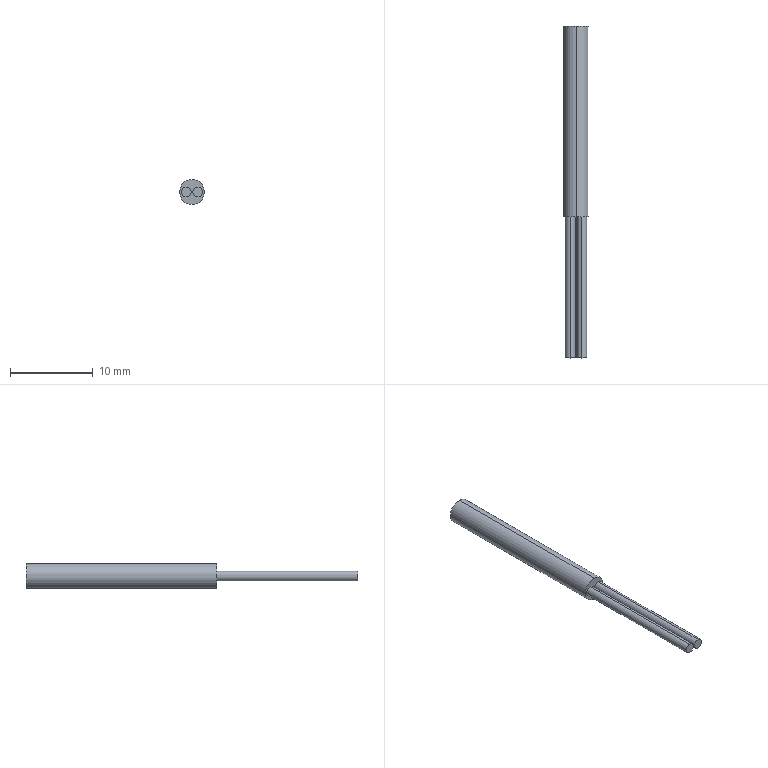Part | STEP file | FU-35FA | 1 solid | 13 faces | box 3 x 40 x 3 mm | volume 201.029 mm3 | cylinder 8 | plane 5 | commonest cylinder face diameters 1.2 x4 1.174 x2 3 x2
STEP:
#1=CARTESIAN_POINT('',(0.,0.,0.));
#2=DIRECTION('',(0.,0.,1.));
#3=DIRECTION('',(1.,0.,0.));
#4=AXIS2_PLACEMENT_3D('',#1,#2,#3);
#5=CARTESIAN_POINT('',(0.,22.999,0.587));
#6=VERTEX_POINT('',#5);
#7=CARTESIAN_POINT('',(0.,23.,0.587));
#8=VERTEX_POINT('',#7);
#9=CARTESIAN_POINT('',(0.,22.999,0.587));
#10=DIRECTION('',(0.,1.,0.));
#11=VECTOR('',#10,1.);
#12=LINE('',#9,#11);
#13=CARTESIAN_POINT('',(0.,22.999,0.));
#14=DIRECTION('',(0.,1.,0.));
#15=DIRECTION('',(0.,0.,1.));
#16=AXIS2_PLACEMENT_3D('',#13,#14,#15);
#17=CYLINDRICAL_SURFACE('',#16,0.587);
#18=CARTESIAN_POINT('',(6.283,0.));
#19=DIRECTION('',(0.,1.));
#20=VECTOR('',#19,1.);
#21=LINE('',#18,#20);
#22=(GEOMETRIC_REPRESENTATION_CONTEXT(2)PARAMETRIC_REPRESENTATION_CONTEXT()REPRESENTATION_CONTEXT('',''));
#23=DEFINITIONAL_REPRESENTATION('',(#21),#22);
#24=PCURVE('',#17,#23);
#25=CARTESIAN_POINT('',(0.,22.999,0.));
#26=DIRECTION('',(0.,1.,0.));
#27=DIRECTION('',(0.,0.,1.));
#28=AXIS2_PLACEMENT_3D('',#25,#26,#27);
#29=CYLINDRICAL_SURFACE('',#28,0.587);
#30=CARTESIAN_POINT('',(0.,0.));
#31=DIRECTION('',(0.,1.));
#32=VECTOR('',#31,1.);
#33=LINE('',#30,#32);
#34=(GEOMETRIC_REPRESENTATION_CONTEXT(2)PARAMETRIC_REPRESENTATION_CONTEXT()REPRESENTATION_CONTEXT('',''));
#35=DEFINITIONAL_REPRESENTATION('',(#33),#34);
#36=PCURVE('',#29,#35);
#37=SURFACE_CURVE('',#12,(#24,#36),.PCURVE_S1.);
#38=EDGE_CURVE('',#6,#8,#37,.T.);
#39=ORIENTED_EDGE('',*,*,#38,.T.);
#40=CARTESIAN_POINT('',(0.,23.,-0.587));
#41=VERTEX_POINT('',#40);
#42=CARTESIAN_POINT('',(0.,23.,0.));
#43=DIRECTION('',(0.,1.,0.));
#44=DIRECTION('',(0.,0.,1.));
#45=AXIS2_PLACEMENT_3D('',#42,#43,#44);
#46=CIRCLE('',#45,0.587);
#47=CARTESIAN_POINT('',(0.,0.001));
#48=DIRECTION('',(1.,0.));
#49=VECTOR('',#48,1.);
#50=LINE('',#47,#49);
#51=(GEOMETRIC_REPRESENTATION_CONTEXT(2)PARAMETRIC_REPRESENTATION_CONTEXT()REPRESENTATION_CONTEXT('',''));
#52=DEFINITIONAL_REPRESENTATION('',(#50),#51);
#53=PCURVE('',#17,#52);
#54=CARTESIAN_POINT('',(0.,23.,0.));
#55=DIRECTION('',(0.,1.,0.));
#56=DIRECTION('',(0.,0.,1.));
#57=AXIS2_PLACEMENT_3D('',#54,#55,#56);
#58=PLANE('',#57);
#59=CARTESIAN_POINT('',(0.,0.));
#60=DIRECTION('',(1.,0.));
#61=AXIS2_PLACEMENT_2D('',#59,#60);
#62=CIRCLE('',#61,0.587);
#63=(GEOMETRIC_REPRESENTATION_CONTEXT(2)PARAMETRIC_REPRESENTATION_CONTEXT()REPRESENTATION_CONTEXT('',''));
#64=DEFINITIONAL_REPRESENTATION('',(#62),#63);
#65=PCURVE('',#58,#64);
#66=SURFACE_CURVE('',#46,(#53,#65),.PCURVE_S1.);
#67=EDGE_CURVE('',#41,#8,#66,.T.);
#68=ORIENTED_EDGE('',*,*,#67,.F.);
#69=CARTESIAN_POINT('',(0.,22.999,-0.587));
#70=VERTEX_POINT('',#69);
#71=CARTESIAN_POINT('',(0.,22.999,-0.587));
#72=DIRECTION('',(0.,1.,0.));
#73=VECTOR('',#72,1.);
#74=LINE('',#71,#73);
#75=CARTESIAN_POINT('',(3.142,0.));
#76=DIRECTION('',(0.,1.));
#77=VECTOR('',#76,1.);
#78=LINE('',#75,#77);
#79=(GEOMETRIC_REPRESENTATION_CONTEXT(2)PARAMETRIC_REPRESENTATION_CONTEXT()REPRESENTATION_CONTEXT('',''));
#80=DEFINITIONAL_REPRESENTATION('',(#78),#79);
#81=PCURVE('',#17,#80);
#82=CARTESIAN_POINT('',(3.142,0.));
#83=DIRECTION('',(0.,1.));
#84=VECTOR('',#83,1.);
#85=LINE('',#82,#84);
#86=(GEOMETRIC_REPRESENTATION_CONTEXT(2)PARAMETRIC_REPRESENTATION_CONTEXT()REPRESENTATION_CONTEXT('',''));
#87=DEFINITIONAL_REPRESENTATION('',(#85),#86);
#88=PCURVE('',#29,#87);
#89=SURFACE_CURVE('',#74,(#81,#88),.PCURVE_S1.);
#90=EDGE_CURVE('',#70,#41,#89,.T.);
#91=ORIENTED_EDGE('',*,*,#90,.F.);
#92=CARTESIAN_POINT('',(0.,22.999,0.));
#93=DIRECTION('',(0.,1.,0.));
#94=DIRECTION('',(0.,0.,1.));
#95=AXIS2_PLACEMENT_3D('',#92,#93,#94);
#96=CIRCLE('',#95,0.587);
#97=CARTESIAN_POINT('',(0.,0.));
#98=DIRECTION('',(1.,0.));
#99=VECTOR('',#98,1.);
#100=LINE('',#97,#99);
#101=(GEOMETRIC_REPRESENTATION_CONTEXT(2)PARAMETRIC_REPRESENTATION_CONTEXT()REPRESENTATION_CONTEXT('',''));
#102=DEFINITIONAL_REPRESENTATION('',(#100),#101);
#103=PCURVE('',#17,#102);
#104=CARTESIAN_POINT('',(0.,22.999,0.));
#105=DIRECTION('',(0.,1.,0.));
#106=DIRECTION('',(0.,0.,1.));
#107=AXIS2_PLACEMENT_3D('',#104,#105,#106);
#108=PLANE('',#107);
#109=CARTESIAN_POINT('',(0.,0.));
#110=DIRECTION('',(1.,0.));
#111=AXIS2_PLACEMENT_2D('',#109,#110);
#112=CIRCLE('',#111,0.587);
#113=(GEOMETRIC_REPRESENTATION_CONTEXT(2)PARAMETRIC_REPRESENTATION_CONTEXT()REPRESENTATION_CONTEXT('',''));
#114=DEFINITIONAL_REPRESENTATION('',(#112),#113);
#115=PCURVE('',#108,#114);
#116=SURFACE_CURVE('',#96,(#103,#115),.PCURVE_S1.);
#117=EDGE_CURVE('',#70,#6,#116,.T.);
#118=ORIENTED_EDGE('',*,*,#117,.T.);
#119=EDGE_LOOP('',(#39,#68,#91,#118));
#120=FACE_BOUND('',#119,.F.);
#121=ADVANCED_FACE('',(#120),#17,.F.);
#122=CARTESIAN_POINT('',(0.7,-17.,-0.6));
#123=VERTEX_POINT('',#122);
#124=CARTESIAN_POINT('',(0.7,-17.,0.6));
#125=VERTEX_POINT('',#124);
#126=CARTESIAN_POINT('',(0.7,-17.,0.));
#127=DIRECTION('',(0.,-1.,0.));
#128=DIRECTION('',(0.,0.,-1.));
#129=AXIS2_PLACEMENT_3D('',#126,#127,#128);
#130=CIRCLE('',#129,0.6);
#131=CARTESIAN_POINT('',(0.7,-17.,0.));
#132=DIRECTION('',(0.,1.,0.));
#133=DIRECTION('',(0.,0.,1.));
#134=AXIS2_PLACEMENT_3D('',#131,#132,#133);
#135=CYLINDRICAL_SURFACE('',#134,0.6);
#136=CARTESIAN_POINT('',(3.142,0.));
#137=DIRECTION('',(-1.,0.));
#138=VECTOR('',#137,1.);
#139=LINE('',#136,#138);
#140=(GEOMETRIC_REPRESENTATION_CONTEXT(2)PARAMETRIC_REPRESENTATION_CONTEXT()REPRESENTATION_CONTEXT('',''));
#141=DEFINITIONAL_REPRESENTATION('',(#139),#140);
#142=PCURVE('',#135,#141);
#143=CARTESIAN_POINT('',(0.7,-17.,0.));
#144=DIRECTION('',(0.,-1.,0.));
#145=DIRECTION('',(0.,0.,-1.));
#146=AXIS2_PLACEMENT_3D('',#143,#144,#145);
#147=PLANE('',#146);
#148=CARTESIAN_POINT('',(0.,0.));
#149=DIRECTION('',(1.,0.));
#150=AXIS2_PLACEMENT_2D('',#148,#149);
#151=CIRCLE('',#150,0.6);
#152=(GEOMETRIC_REPRESENTATION_CONTEXT(2)PARAMETRIC_REPRESENTATION_CONTEXT()REPRESENTATION_CONTEXT('',''));
#153=DEFINITIONAL_REPRESENTATION('',(#151),#152);
#154=PCURVE('',#147,#153);
#155=SURFACE_CURVE('',#130,(#142,#154),.PCURVE_S1.);
#156=EDGE_CURVE('',#123,#125,#155,.T.);
#157=ORIENTED_EDGE('',*,*,#156,.F.);
#158=CARTESIAN_POINT('',(0.7,0.,-0.6));
#159=VERTEX_POINT('',#158);
#160=CARTESIAN_POINT('',(0.7,-17.,-0.6));
#161=DIRECTION('',(0.,1.,0.));
#162=VECTOR('',#161,1.);
#163=LINE('',#160,#162);
#164=CARTESIAN_POINT('',(3.142,0.));
#165=DIRECTION('',(0.,1.));
#166=VECTOR('',#165,1.);
#167=LINE('',#164,#166);
#168=(GEOMETRIC_REPRESENTATION_CONTEXT(2)PARAMETRIC_REPRESENTATION_CONTEXT()REPRESENTATION_CONTEXT('',''));
#169=DEFINITIONAL_REPRESENTATION('',(#167),#168);
#170=PCURVE('',#135,#169);
#171=CARTESIAN_POINT('',(0.7,-17.,0.));
#172=DIRECTION('',(0.,1.,0.));
#173=DIRECTION('',(0.,0.,1.));
#174=AXIS2_PLACEMENT_3D('',#171,#172,#173);
#175=CYLINDRICAL_SURFACE('',#174,0.6);
#176=CARTESIAN_POINT('',(3.142,0.));
#177=DIRECTION('',(0.,1.));
#178=VECTOR('',#177,1.);
#179=LINE('',#176,#178);
#180=(GEOMETRIC_REPRESENTATION_CONTEXT(2)PARAMETRIC_REPRESENTATION_CONTEXT()REPRESENTATION_CONTEXT('',''));
#181=DEFINITIONAL_REPRESENTATION('',(#179),#180);
#182=PCURVE('',#175,#181);
#183=SURFACE_CURVE('',#163,(#170,#182),.PCURVE_S1.);
#184=EDGE_CURVE('',#123,#159,#183,.T.);
#185=ORIENTED_EDGE('',*,*,#184,.T.);
#186=CARTESIAN_POINT('',(0.7,0.,0.6));
#187=VERTEX_POINT('',#186);
#188=CARTESIAN_POINT('',(0.7,0.,0.));
#189=DIRECTION('',(0.,-1.,0.));
#190=DIRECTION('',(0.,0.,1.));
#191=AXIS2_PLACEMENT_3D('',#188,#189,#190);
#192=CIRCLE('',#191,0.6);
#193=CARTESIAN_POINT('',(6.283,17.));
#194=DIRECTION('',(-1.,0.));
#195=VECTOR('',#194,1.);
#196=LINE('',#193,#195);
#197=(GEOMETRIC_REPRESENTATION_CONTEXT(2)PARAMETRIC_REPRESENTATION_CONTEXT()REPRESENTATION_CONTEXT('',''));
#198=DEFINITIONAL_REPRESENTATION('',(#196),#197);
#199=PCURVE('',#135,#198);
#200=CARTESIAN_POINT('',(0.,0.,0.));
#201=DIRECTION('',(0.,1.,0.));
#202=DIRECTION('',(0.,0.,1.));
#203=AXIS2_PLACEMENT_3D('',#200,#201,#202);
#204=PLANE('',#203);
#205=CARTESIAN_POINT('',(0.6,0.7));
#206=CARTESIAN_POINT('',(0.6,-0.3392));
#207=CARTESIAN_POINT('',(-0.3,0.1804));
#208=CARTESIAN_POINT('',(-1.2,0.7));
#209=CARTESIAN_POINT('',(-0.3,1.22));
#210=CARTESIAN_POINT('',(0.6,1.739));
#211=CARTESIAN_POINT('',(0.6,0.7));
#212=(BOUNDED_CURVE()B_SPLINE_CURVE(2,(#205,#206,#207,#208,#209,#210,#211),.UNSPECIFIED.,.T.,.F.)B_SPLINE_CURVE_WITH_KNOTS((1,2,2,2,2,1),(-2.094,0.,2.094,4.189,6.283,8.378),.UNSPECIFIED.)CURVE()GEOMETRIC_REPRESENTATION_ITEM()RATIONAL_B_SPLINE_CURVE((1.,0.5,1.,0.5,1.,0.5,1.))REPRESENTATION_ITEM(''));
#213=(GEOMETRIC_REPRESENTATION_CONTEXT(2)PARAMETRIC_REPRESENTATION_CONTEXT()REPRESENTATION_CONTEXT('',''));
#214=DEFINITIONAL_REPRESENTATION('',(#212),#213);
#215=PCURVE('',#204,#214);
#216=SURFACE_CURVE('',#192,(#199,#215),.PCURVE_S1.);
#217=EDGE_CURVE('',#159,#187,#216,.T.);
#218=ORIENTED_EDGE('',*,*,#217,.T.);
#219=CARTESIAN_POINT('',(0.7,-17.,0.6));
#220=DIRECTION('',(0.,1.,0.));
#221=VECTOR('',#220,1.);
#222=LINE('',#219,#221);
#223=CARTESIAN_POINT('',(0.,0.));
#224=DIRECTION('',(0.,1.));
#225=VECTOR('',#224,1.);
#226=LINE('',#223,#225);
#227=(GEOMETRIC_REPRESENTATION_CONTEXT(2)PARAMETRIC_REPRESENTATION_CONTEXT()REPRESENTATION_CONTEXT('',''));
#228=DEFINITIONAL_REPRESENTATION('',(#226),#227);
#229=PCURVE('',#135,#228);
#230=CARTESIAN_POINT('',(6.283,0.));
#231=DIRECTION('',(0.,1.));
#232=VECTOR('',#231,1.);
#233=LINE('',#230,#232);
#234=(GEOMETRIC_REPRESENTATION_CONTEXT(2)PARAMETRIC_REPRESENTATION_CONTEXT()REPRESENTATION_CONTEXT('',''));
#235=DEFINITIONAL_REPRESENTATION('',(#233),#234);
#236=PCURVE('',#175,#235);
#237=SURFACE_CURVE('',#222,(#229,#236),.PCURVE_S1.);
#238=EDGE_CURVE('',#125,#187,#237,.T.);
#239=ORIENTED_EDGE('',*,*,#238,.F.);
#240=EDGE_LOOP('',(#157,#185,#218,#239));
#241=FACE_BOUND('',#240,.T.);
#242=ADVANCED_FACE('',(#241),#135,.T.);
#243=CARTESIAN_POINT('',(-0.7,-17.,-0.6));
#244=VERTEX_POINT('',#243);
#245=CARTESIAN_POINT('',(-0.7,-17.,0.6));
#246=VERTEX_POINT('',#245);
#247=CARTESIAN_POINT('',(-0.7,-17.,0.));
#248=DIRECTION('',(0.,-1.,0.));
#249=DIRECTION('',(0.,0.,-1.));
#250=AXIS2_PLACEMENT_3D('',#247,#248,#249);
#251=CIRCLE('',#250,0.6);
#252=CARTESIAN_POINT('',(-0.7,-17.,0.));
#253=DIRECTION('',(0.,1.,0.));
#254=DIRECTION('',(0.,0.,1.));
#255=AXIS2_PLACEMENT_3D('',#252,#253,#254);
#256=CYLINDRICAL_SURFACE('',#255,0.6);
#257=CARTESIAN_POINT('',(3.142,0.));
#258=DIRECTION('',(-1.,0.));
#259=VECTOR('',#258,1.);
#260=LINE('',#257,#259);
#261=(GEOMETRIC_REPRESENTATION_CONTEXT(2)PARAMETRIC_REPRESENTATION_CONTEXT()REPRESENTATION_CONTEXT('',''));
#262=DEFINITIONAL_REPRESENTATION('',(#260),#261);
#263=PCURVE('',#256,#262);
#264=CARTESIAN_POINT('',(-0.7,-17.,0.));
#265=DIRECTION('',(0.,-1.,0.));
#266=DIRECTION('',(0.,0.,-1.));
#267=AXIS2_PLACEMENT_3D('',#264,#265,#266);
#268=PLANE('',#267);
#269=CARTESIAN_POINT('',(0.,0.));
#270=DIRECTION('',(1.,0.));
#271=AXIS2_PLACEMENT_2D('',#269,#270);
#272=CIRCLE('',#271,0.6);
#273=(GEOMETRIC_REPRESENTATION_CONTEXT(2)PARAMETRIC_REPRESENTATION_CONTEXT()REPRESENTATION_CONTEXT('',''));
#274=DEFINITIONAL_REPRESENTATION('',(#272),#273);
#275=PCURVE('',#268,#274);
#276=SURFACE_CURVE('',#251,(#263,#275),.PCURVE_S1.);
#277=EDGE_CURVE('',#244,#246,#276,.T.);
#278=ORIENTED_EDGE('',*,*,#277,.F.);
#279=CARTESIAN_POINT('',(-0.7,0.,-0.6));
#280=VERTEX_POINT('',#279);
#281=CARTESIAN_POINT('',(-0.7,-17.,-0.6));
#282=DIRECTION('',(0.,1.,0.));
#283=VECTOR('',#282,1.);
#284=LINE('',#281,#283);
#285=CARTESIAN_POINT('',(3.142,0.));
#286=DIRECTION('',(0.,1.));
#287=VECTOR('',#286,1.);
#288=LINE('',#285,#287);
#289=(GEOMETRIC_REPRESENTATION_CONTEXT(2)PARAMETRIC_REPRESENTATION_CONTEXT()REPRESENTATION_CONTEXT('',''));
#290=DEFINITIONAL_REPRESENTATION('',(#288),#289);
#291=PCURVE('',#256,#290);
#292=CARTESIAN_POINT('',(-0.7,-17.,0.));
#293=DIRECTION('',(0.,1.,0.));
#294=DIRECTION('',(0.,0.,1.));
#295=AXIS2_PLACEMENT_3D('',#292,#293,#294);
#296=CYLINDRICAL_SURFACE('',#295,0.6);
#297=CARTESIAN_POINT('',(3.142,0.));
#298=DIRECTION('',(0.,1.));
#299=VECTOR('',#298,1.);
#300=LINE('',#297,#299);
#301=(GEOMETRIC_REPRESENTATION_CONTEXT(2)PARAMETRIC_REPRESENTATION_CONTEXT()REPRESENTATION_CONTEXT('',''));
#302=DEFINITIONAL_REPRESENTATION('',(#300),#301);
#303=PCURVE('',#296,#302);
#304=SURFACE_CURVE('',#284,(#291,#303),.PCURVE_S1.);
#305=EDGE_CURVE('',#244,#280,#304,.T.);
#306=ORIENTED_EDGE('',*,*,#305,.T.);
#307=CARTESIAN_POINT('',(-0.7,0.,0.6));
#308=VERTEX_POINT('',#307);
#309=CARTESIAN_POINT('',(-0.7,0.,0.));
#310=DIRECTION('',(0.,-1.,0.));
#311=DIRECTION('',(0.,0.,1.));
#312=AXIS2_PLACEMENT_3D('',#309,#310,#311);
#313=CIRCLE('',#312,0.6);
#314=CARTESIAN_POINT('',(6.283,17.));
#315=DIRECTION('',(-1.,0.));
#316=VECTOR('',#315,1.);
#317=LINE('',#314,#316);
#318=(GEOMETRIC_REPRESENTATION_CONTEXT(2)PARAMETRIC_REPRESENTATION_CONTEXT()REPRESENTATION_CONTEXT('',''));
#319=DEFINITIONAL_REPRESENTATION('',(#317),#318);
#320=PCURVE('',#256,#319);
#321=CARTESIAN_POINT('',(0.6,-0.7));
#322=CARTESIAN_POINT('',(0.6,-1.739));
#323=CARTESIAN_POINT('',(-0.3,-1.22));
#324=CARTESIAN_POINT('',(-1.2,-0.7));
#325=CARTESIAN_POINT('',(-0.3,-0.1804));
#326=CARTESIAN_POINT('',(0.6,0.3392));
#327=CARTESIAN_POINT('',(0.6,-0.7));
#328=(BOUNDED_CURVE()B_SPLINE_CURVE(2,(#321,#322,#323,#324,#325,#326,#327),.UNSPECIFIED.,.T.,.F.)B_SPLINE_CURVE_WITH_KNOTS((1,2,2,2,2,1),(-2.094,0.,2.094,4.189,6.283,8.378),.UNSPECIFIED.)CURVE()GEOMETRIC_REPRESENTATION_ITEM()RATIONAL_B_SPLINE_CURVE((1.,0.5,1.,0.5,1.,0.5,1.))REPRESENTATION_ITEM(''));
#329=(GEOMETRIC_REPRESENTATION_CONTEXT(2)PARAMETRIC_REPRESENTATION_CONTEXT()REPRESENTATION_CONTEXT('',''));
#330=DEFINITIONAL_REPRESENTATION('',(#328),#329);
#331=PCURVE('',#204,#330);
#332=SURFACE_CURVE('',#313,(#320,#331),.PCURVE_S1.);
#333=EDGE_CURVE('',#280,#308,#332,.T.);
#334=ORIENTED_EDGE('',*,*,#333,.T.);
#335=CARTESIAN_POINT('',(-0.7,-17.,0.6));
#336=DIRECTION('',(0.,1.,0.));
#337=VECTOR('',#336,1.);
#338=LINE('',#335,#337);
#339=CARTESIAN_POINT('',(0.,0.));
#340=DIRECTION('',(0.,1.));
#341=VECTOR('',#340,1.);
#342=LINE('',#339,#341);
#343=(GEOMETRIC_REPRESENTATION_CONTEXT(2)PARAMETRIC_REPRESENTATION_CONTEXT()REPRESENTATION_CONTEXT('',''));
#344=DEFINITIONAL_REPRESENTATION('',(#342),#343);
#345=PCURVE('',#256,#344);
#346=CARTESIAN_POINT('',(6.283,0.));
#347=DIRECTION('',(0.,1.));
#348=VECTOR('',#347,1.);
#349=LINE('',#346,#348);
#350=(GEOMETRIC_REPRESENTATION_CONTEXT(2)PARAMETRIC_REPRESENTATION_CONTEXT()REPRESENTATION_CONTEXT('',''));
#351=DEFINITIONAL_REPRESENTATION('',(#349),#350);
#352=PCURVE('',#296,#351);
#353=SURFACE_CURVE('',#338,(#345,#352),.PCURVE_S1.);
#354=EDGE_CURVE('',#246,#308,#353,.T.);
#355=ORIENTED_EDGE('',*,*,#354,.F.);
#356=EDGE_LOOP('',(#278,#306,#334,#355));
#357=FACE_BOUND('',#356,.T.);
#358=ADVANCED_FACE('',(#357),#256,.T.);
#359=CARTESIAN_POINT('',(0.,23.,1.5));
#360=VERTEX_POINT('',#359);
#361=CARTESIAN_POINT('',(0.,23.,-1.5));
#362=VERTEX_POINT('',#361);
#363=CARTESIAN_POINT('',(0.,23.,0.));
#364=DIRECTION('',(0.,1.,0.));
#365=DIRECTION('',(0.,0.,1.));
#366=AXIS2_PLACEMENT_3D('',#363,#364,#365);
#367=CIRCLE('',#366,1.5);
#368=CARTESIAN_POINT('',(0.,23.,0.));
#369=DIRECTION('',(0.,-1.,0.));
#370=DIRECTION('',(0.,0.,-1.));
#371=AXIS2_PLACEMENT_3D('',#368,#369,#370);
#372=CYLINDRICAL_SURFACE('',#371,1.5);
#373=CARTESIAN_POINT('',(3.142,0.));
#374=DIRECTION('',(-1.,0.));
#375=VECTOR('',#374,1.);
#376=LINE('',#373,#375);
#377=(GEOMETRIC_REPRESENTATION_CONTEXT(2)PARAMETRIC_REPRESENTATION_CONTEXT()REPRESENTATION_CONTEXT('',''));
#378=DEFINITIONAL_REPRESENTATION('',(#376),#377);
#379=PCURVE('',#372,#378);
#380=CARTESIAN_POINT('',(0.,0.));
#381=DIRECTION('',(1.,0.));
#382=AXIS2_PLACEMENT_2D('',#380,#381);
#383=CIRCLE('',#382,1.5);
#384=(GEOMETRIC_REPRESENTATION_CONTEXT(2)PARAMETRIC_REPRESENTATION_CONTEXT()REPRESENTATION_CONTEXT('',''));
#385=DEFINITIONAL_REPRESENTATION('',(#383),#384);
#386=PCURVE('',#58,#385);
#387=SURFACE_CURVE('',#367,(#379,#386),.PCURVE_S1.);
#388=EDGE_CURVE('',#360,#362,#387,.T.);
#389=ORIENTED_EDGE('',*,*,#388,.F.);
#390=CARTESIAN_POINT('',(0.,0.,1.5));
#391=VERTEX_POINT('',#390);
#392=CARTESIAN_POINT('',(0.,23.,1.5));
#393=DIRECTION('',(0.,-1.,0.));
#394=VECTOR('',#393,1.);
#395=LINE('',#392,#394);
#396=CARTESIAN_POINT('',(3.142,0.));
#397=DIRECTION('',(0.,1.));
#398=VECTOR('',#397,1.);
#399=LINE('',#396,#398);
#400=(GEOMETRIC_REPRESENTATION_CONTEXT(2)PARAMETRIC_REPRESENTATION_CONTEXT()REPRESENTATION_CONTEXT('',''));
#401=DEFINITIONAL_REPRESENTATION('',(#399),#400);
#402=PCURVE('',#372,#401);
#403=CARTESIAN_POINT('',(0.,23.,0.));
#404=DIRECTION('',(0.,-1.,0.));
#405=DIRECTION('',(0.,0.,-1.));
#406=AXIS2_PLACEMENT_3D('',#403,#404,#405);
#407=CYLINDRICAL_SURFACE('',#406,1.5);
#408=CARTESIAN_POINT('',(3.142,0.));
#409=DIRECTION('',(0.,1.));
#410=VECTOR('',#409,1.);
#411=LINE('',#408,#410);
#412=(GEOMETRIC_REPRESENTATION_CONTEXT(2)PARAMETRIC_REPRESENTATION_CONTEXT()REPRESENTATION_CONTEXT('',''));
#413=DEFINITIONAL_REPRESENTATION('',(#411),#412);
#414=PCURVE('',#407,#413);
#415=SURFACE_CURVE('',#395,(#402,#414),.PCURVE_S1.);
#416=EDGE_CURVE('',#360,#391,#415,.T.);
#417=ORIENTED_EDGE('',*,*,#416,.T.);
#418=CARTESIAN_POINT('',(0.,0.,-1.5));
#419=VERTEX_POINT('',#418);
#420=CARTESIAN_POINT('',(0.,0.,0.));
#421=DIRECTION('',(0.,1.,0.));
#422=DIRECTION('',(0.,0.,1.));
#423=AXIS2_PLACEMENT_3D('',#420,#421,#422);
#424=CIRCLE('',#423,1.5);
#425=CARTESIAN_POINT('',(3.142,23.));
#426=DIRECTION('',(-1.,0.));
#427=VECTOR('',#426,1.);
#428=LINE('',#425,#427);
#429=(GEOMETRIC_REPRESENTATION_CONTEXT(2)PARAMETRIC_REPRESENTATION_CONTEXT()REPRESENTATION_CONTEXT('',''));
#430=DEFINITIONAL_REPRESENTATION('',(#428),#429);
#431=PCURVE('',#372,#430);
#432=CARTESIAN_POINT('',(0.,0.));
#433=DIRECTION('',(1.,0.));
#434=AXIS2_PLACEMENT_2D('',#432,#433);
#435=CIRCLE('',#434,1.5);
#436=(GEOMETRIC_REPRESENTATION_CONTEXT(2)PARAMETRIC_REPRESENTATION_CONTEXT()REPRESENTATION_CONTEXT('',''));
#437=DEFINITIONAL_REPRESENTATION('',(#435),#436);
#438=PCURVE('',#204,#437);
#439=SURFACE_CURVE('',#424,(#431,#438),.PCURVE_S1.);
#440=EDGE_CURVE('',#391,#419,#439,.T.);
#441=ORIENTED_EDGE('',*,*,#440,.T.);
#442=CARTESIAN_POINT('',(0.,23.,-1.5));
#443=DIRECTION('',(0.,-1.,0.));
#444=VECTOR('',#443,1.);
#445=LINE('',#442,#444);
#446=CARTESIAN_POINT('',(0.,0.));
#447=DIRECTION('',(0.,1.));
#448=VECTOR('',#447,1.);
#449=LINE('',#446,#448);
#450=(GEOMETRIC_REPRESENTATION_CONTEXT(2)PARAMETRIC_REPRESENTATION_CONTEXT()REPRESENTATION_CONTEXT('',''));
#451=DEFINITIONAL_REPRESENTATION('',(#449),#450);
#452=PCURVE('',#372,#451);
#453=CARTESIAN_POINT('',(6.283,0.));
#454=DIRECTION('',(0.,1.));
#455=VECTOR('',#454,1.);
#456=LINE('',#453,#455);
#457=(GEOMETRIC_REPRESENTATION_CONTEXT(2)PARAMETRIC_REPRESENTATION_CONTEXT()REPRESENTATION_CONTEXT('',''));
#458=DEFINITIONAL_REPRESENTATION('',(#456),#457);
#459=PCURVE('',#407,#458);
#460=SURFACE_CURVE('',#445,(#452,#459),.PCURVE_S1.);
#461=EDGE_CURVE('',#362,#419,#460,.T.);
#462=ORIENTED_EDGE('',*,*,#461,.F.);
#463=EDGE_LOOP('',(#389,#417,#441,#462));
#464=FACE_BOUND('',#463,.T.);
#465=ADVANCED_FACE('',(#464),#372,.T.);
#466=CARTESIAN_POINT('',(-0.7,0.,0.));
#467=DIRECTION('',(0.,-1.,0.));
#468=DIRECTION('',(0.,0.,1.));
#469=AXIS2_PLACEMENT_3D('',#466,#467,#468);
#470=CIRCLE('',#469,0.6);
#471=CARTESIAN_POINT('',(0.6,-0.7));
#472=CARTESIAN_POINT('',(0.6,-1.739));
#473=CARTESIAN_POINT('',(-0.3,-1.22));
#474=CARTESIAN_POINT('',(-1.2,-0.7));
#475=CARTESIAN_POINT('',(-0.3,-0.1804));
#476=CARTESIAN_POINT('',(0.6,0.3392));
#477=CARTESIAN_POINT('',(0.6,-0.7));
#478=(BOUNDED_CURVE()B_SPLINE_CURVE(2,(#471,#472,#473,#474,#475,#476,#477),.UNSPECIFIED.,.T.,.F.)B_SPLINE_CURVE_WITH_KNOTS((1,2,2,2,2,1),(-2.094,0.,2.094,4.189,6.283,8.378),.UNSPECIFIED.)CURVE()GEOMETRIC_REPRESENTATION_ITEM()RATIONAL_B_SPLINE_CURVE((1.,0.5,1.,0.5,1.,0.5,1.))REPRESENTATION_ITEM(''));
#479=(GEOMETRIC_REPRESENTATION_CONTEXT(2)PARAMETRIC_REPRESENTATION_CONTEXT()REPRESENTATION_CONTEXT('',''));
#480=DEFINITIONAL_REPRESENTATION('',(#478),#479);
#481=PCURVE('',#204,#480);
#482=CARTESIAN_POINT('',(6.283,17.));
#483=DIRECTION('',(-1.,0.));
#484=VECTOR('',#483,1.);
#485=LINE('',#482,#484);
#486=(GEOMETRIC_REPRESENTATION_CONTEXT(2)PARAMETRIC_REPRESENTATION_CONTEXT()REPRESENTATION_CONTEXT('',''));
#487=DEFINITIONAL_REPRESENTATION('',(#485),#486);
#488=PCURVE('',#296,#487);
#489=SURFACE_CURVE('',#470,(#481,#488),.PCURVE_S1.);
#490=EDGE_CURVE('',#308,#280,#489,.T.);
#491=ORIENTED_EDGE('',*,*,#490,.F.);
#492=ORIENTED_EDGE('',*,*,#333,.F.);
#493=EDGE_LOOP('',(#491,#492));
#494=FACE_BOUND('',#493,.T.);
#495=CARTESIAN_POINT('',(0.,0.,0.));
#496=DIRECTION('',(0.,1.,0.));
#497=DIRECTION('',(0.,0.,1.));
#498=AXIS2_PLACEMENT_3D('',#495,#496,#497);
#499=CIRCLE('',#498,1.5);
#500=CARTESIAN_POINT('',(0.,0.));
#501=DIRECTION('',(1.,0.));
#502=AXIS2_PLACEMENT_2D('',#500,#501);
#503=CIRCLE('',#502,1.5);
#504=(GEOMETRIC_REPRESENTATION_CONTEXT(2)PARAMETRIC_REPRESENTATION_CONTEXT()REPRESENTATION_CONTEXT('',''));
#505=DEFINITIONAL_REPRESENTATION('',(#503),#504);
#506=PCURVE('',#204,#505);
#507=CARTESIAN_POINT('',(9.425,23.));
#508=DIRECTION('',(-1.,0.));
#509=VECTOR('',#508,1.);
#510=LINE('',#507,#509);
#511=(GEOMETRIC_REPRESENTATION_CONTEXT(2)PARAMETRIC_REPRESENTATION_CONTEXT()REPRESENTATION_CONTEXT('',''));
#512=DEFINITIONAL_REPRESENTATION('',(#510),#511);
#513=PCURVE('',#407,#512);
#514=SURFACE_CURVE('',#499,(#506,#513),.PCURVE_S1.);
#515=EDGE_CURVE('',#419,#391,#514,.T.);
#516=ORIENTED_EDGE('',*,*,#515,.F.);
#517=ORIENTED_EDGE('',*,*,#440,.F.);
#518=EDGE_LOOP('',(#516,#517));
#519=FACE_BOUND('',#518,.T.);
#520=CARTESIAN_POINT('',(0.7,0.,0.));
#521=DIRECTION('',(0.,-1.,0.));
#522=DIRECTION('',(0.,0.,1.));
#523=AXIS2_PLACEMENT_3D('',#520,#521,#522);
#524=CIRCLE('',#523,0.6);
#525=CARTESIAN_POINT('',(0.6,0.7));
#526=CARTESIAN_POINT('',(0.6,-0.3392));
#527=CARTESIAN_POINT('',(-0.3,0.1804));
#528=CARTESIAN_POINT('',(-1.2,0.7));
#529=CARTESIAN_POINT('',(-0.3,1.22));
#530=CARTESIAN_POINT('',(0.6,1.739));
#531=CARTESIAN_POINT('',(0.6,0.7));
#532=(BOUNDED_CURVE()B_SPLINE_CURVE(2,(#525,#526,#527,#528,#529,#530,#531),.UNSPECIFIED.,.T.,.F.)B_SPLINE_CURVE_WITH_KNOTS((1,2,2,2,2,1),(-2.094,0.,2.094,4.189,6.283,8.378),.UNSPECIFIED.)CURVE()GEOMETRIC_REPRESENTATION_ITEM()RATIONAL_B_SPLINE_CURVE((1.,0.5,1.,0.5,1.,0.5,1.))REPRESENTATION_ITEM(''));
#533=(GEOMETRIC_REPRESENTATION_CONTEXT(2)PARAMETRIC_REPRESENTATION_CONTEXT()REPRESENTATION_CONTEXT('',''));
#534=DEFINITIONAL_REPRESENTATION('',(#532),#533);
#535=PCURVE('',#204,#534);
#536=CARTESIAN_POINT('',(6.283,17.));
#537=DIRECTION('',(-1.,0.));
#538=VECTOR('',#537,1.);
#539=LINE('',#536,#538);
#540=(GEOMETRIC_REPRESENTATION_CONTEXT(2)PARAMETRIC_REPRESENTATION_CONTEXT()REPRESENTATION_CONTEXT('',''));
#541=DEFINITIONAL_REPRESENTATION('',(#539),#540);
#542=PCURVE('',#175,#541);
#543=SURFACE_CURVE('',#524,(#535,#542),.PCURVE_S1.);
#544=EDGE_CURVE('',#187,#159,#543,.T.);
#545=ORIENTED_EDGE('',*,*,#544,.F.);
#546=ORIENTED_EDGE('',*,*,#217,.F.);
#547=EDGE_LOOP('',(#545,#546));
#548=FACE_BOUND('',#547,.T.);
#549=ADVANCED_FACE('',(#494,#519,#548),#204,.F.);
#550=ORIENTED_EDGE('',*,*,#416,.F.);
#551=CARTESIAN_POINT('',(0.,23.,0.));
#552=DIRECTION('',(0.,1.,0.));
#553=DIRECTION('',(0.,0.,1.));
#554=AXIS2_PLACEMENT_3D('',#551,#552,#553);
#555=CIRCLE('',#554,1.5);
#556=CARTESIAN_POINT('',(9.425,0.));
#557=DIRECTION('',(-1.,0.));
#558=VECTOR('',#557,1.);
#559=LINE('',#556,#558);
#560=(GEOMETRIC_REPRESENTATION_CONTEXT(2)PARAMETRIC_REPRESENTATION_CONTEXT()REPRESENTATION_CONTEXT('',''));
#561=DEFINITIONAL_REPRESENTATION('',(#559),#560);
#562=PCURVE('',#407,#561);
#563=CARTESIAN_POINT('',(0.,0.));
#564=DIRECTION('',(1.,0.));
#565=AXIS2_PLACEMENT_2D('',#563,#564);
#566=CIRCLE('',#565,1.5);
#567=(GEOMETRIC_REPRESENTATION_CONTEXT(2)PARAMETRIC_REPRESENTATION_CONTEXT()REPRESENTATION_CONTEXT('',''));
#568=DEFINITIONAL_REPRESENTATION('',(#566),#567);
#569=PCURVE('',#58,#568);
#570=SURFACE_CURVE('',#555,(#562,#569),.PCURVE_S1.);
#571=EDGE_CURVE('',#362,#360,#570,.T.);
#572=ORIENTED_EDGE('',*,*,#571,.F.);
#573=ORIENTED_EDGE('',*,*,#461,.T.);
#574=ORIENTED_EDGE('',*,*,#515,.T.);
#575=EDGE_LOOP('',(#550,#572,#573,#574));
#576=FACE_BOUND('',#575,.T.);
#577=ADVANCED_FACE('',(#576),#407,.T.);
#578=CARTESIAN_POINT('',(0.,23.,0.));
#579=DIRECTION('',(0.,1.,0.));
#580=DIRECTION('',(0.,0.,1.));
#581=AXIS2_PLACEMENT_3D('',#578,#579,#580);
#582=CIRCLE('',#581,0.587);
#583=CARTESIAN_POINT('',(0.,0.));
#584=DIRECTION('',(1.,0.));
#585=AXIS2_PLACEMENT_2D('',#583,#584);
#586=CIRCLE('',#585,0.587);
#587=(GEOMETRIC_REPRESENTATION_CONTEXT(2)PARAMETRIC_REPRESENTATION_CONTEXT()REPRESENTATION_CONTEXT('',''));
#588=DEFINITIONAL_REPRESENTATION('',(#586),#587);
#589=PCURVE('',#58,#588);
#590=CARTESIAN_POINT('',(0.,0.001));
#591=DIRECTION('',(1.,0.));
#592=VECTOR('',#591,1.);
#593=LINE('',#590,#592);
#594=(GEOMETRIC_REPRESENTATION_CONTEXT(2)PARAMETRIC_REPRESENTATION_CONTEXT()REPRESENTATION_CONTEXT('',''));
#595=DEFINITIONAL_REPRESENTATION('',(#593),#594);
#596=PCURVE('',#29,#595);
#597=SURFACE_CURVE('',#582,(#589,#596),.PCURVE_S1.);
#598=EDGE_CURVE('',#8,#41,#597,.T.);
#599=ORIENTED_EDGE('',*,*,#598,.F.);
#600=ORIENTED_EDGE('',*,*,#67,.F.);
#601=EDGE_LOOP('',(#599,#600));
#602=FACE_BOUND('',#601,.T.);
#603=ORIENTED_EDGE('',*,*,#571,.T.);
#604=ORIENTED_EDGE('',*,*,#388,.T.);
#605=EDGE_LOOP('',(#603,#604));
#606=FACE_BOUND('',#605,.T.);
#607=ADVANCED_FACE('',(#602,#606),#58,.T.);
#608=ORIENTED_EDGE('',*,*,#305,.F.);
#609=CARTESIAN_POINT('',(-0.7,-17.,0.));
#610=DIRECTION('',(0.,-1.,0.));
#611=DIRECTION('',(0.,0.,-1.));
#612=AXIS2_PLACEMENT_3D('',#609,#610,#611);
#613=CIRCLE('',#612,0.6);
#614=CARTESIAN_POINT('',(9.425,0.));
#615=DIRECTION('',(-1.,0.));
#616=VECTOR('',#615,1.);
#617=LINE('',#614,#616);
#618=(GEOMETRIC_REPRESENTATION_CONTEXT(2)PARAMETRIC_REPRESENTATION_CONTEXT()REPRESENTATION_CONTEXT('',''));
#619=DEFINITIONAL_REPRESENTATION('',(#617),#618);
#620=PCURVE('',#296,#619);
#621=CARTESIAN_POINT('',(0.,0.));
#622=DIRECTION('',(1.,0.));
#623=AXIS2_PLACEMENT_2D('',#621,#622);
#624=CIRCLE('',#623,0.6);
#625=(GEOMETRIC_REPRESENTATION_CONTEXT(2)PARAMETRIC_REPRESENTATION_CONTEXT()REPRESENTATION_CONTEXT('',''));
#626=DEFINITIONAL_REPRESENTATION('',(#624),#625);
#627=PCURVE('',#268,#626);
#628=SURFACE_CURVE('',#613,(#620,#627),.PCURVE_S1.);
#629=EDGE_CURVE('',#246,#244,#628,.T.);
#630=ORIENTED_EDGE('',*,*,#629,.F.);
#631=ORIENTED_EDGE('',*,*,#354,.T.);
#632=ORIENTED_EDGE('',*,*,#490,.T.);
#633=EDGE_LOOP('',(#608,#630,#631,#632));
#634=FACE_BOUND('',#633,.T.);
#635=ADVANCED_FACE('',(#634),#296,.T.);
#636=ORIENTED_EDGE('',*,*,#629,.T.);
#637=ORIENTED_EDGE('',*,*,#277,.T.);
#638=EDGE_LOOP('',(#636,#637));
#639=FACE_BOUND('',#638,.T.);
#640=ADVANCED_FACE('',(#639),#268,.T.);
#641=ORIENTED_EDGE('',*,*,#184,.F.);
#642=CARTESIAN_POINT('',(0.7,-17.,0.));
#643=DIRECTION('',(0.,-1.,0.));
#644=DIRECTION('',(0.,0.,-1.));
#645=AXIS2_PLACEMENT_3D('',#642,#643,#644);
#646=CIRCLE('',#645,0.6);
#647=CARTESIAN_POINT('',(9.425,0.));
#648=DIRECTION('',(-1.,0.));
#649=VECTOR('',#648,1.);
#650=LINE('',#647,#649);
#651=(GEOMETRIC_REPRESENTATION_CONTEXT(2)PARAMETRIC_REPRESENTATION_CONTEXT()REPRESENTATION_CONTEXT('',''));
#652=DEFINITIONAL_REPRESENTATION('',(#650),#651);
#653=PCURVE('',#175,#652);
#654=CARTESIAN_POINT('',(0.,0.));
#655=DIRECTION('',(1.,0.));
#656=AXIS2_PLACEMENT_2D('',#654,#655);
#657=CIRCLE('',#656,0.6);
#658=(GEOMETRIC_REPRESENTATION_CONTEXT(2)PARAMETRIC_REPRESENTATION_CONTEXT()REPRESENTATION_CONTEXT('',''));
#659=DEFINITIONAL_REPRESENTATION('',(#657),#658);
#660=PCURVE('',#147,#659);
#661=SURFACE_CURVE('',#646,(#653,#660),.PCURVE_S1.);
#662=EDGE_CURVE('',#125,#123,#661,.T.);
#663=ORIENTED_EDGE('',*,*,#662,.F.);
#664=ORIENTED_EDGE('',*,*,#238,.T.);
#665=ORIENTED_EDGE('',*,*,#544,.T.);
#666=EDGE_LOOP('',(#641,#663,#664,#665));
#667=FACE_BOUND('',#666,.T.);
#668=ADVANCED_FACE('',(#667),#175,.T.);
#669=ORIENTED_EDGE('',*,*,#662,.T.);
#670=ORIENTED_EDGE('',*,*,#156,.T.);
#671=EDGE_LOOP('',(#669,#670));
#672=FACE_BOUND('',#671,.T.);
#673=ADVANCED_FACE('',(#672),#147,.T.);
#674=ORIENTED_EDGE('',*,*,#598,.F.);
#675=ORIENTED_EDGE('',*,*,#38,.F.);
#676=CARTESIAN_POINT('',(0.,22.999,0.));
#677=DIRECTION('',(0.,1.,0.));
#678=DIRECTION('',(0.,0.,1.));
#679=AXIS2_PLACEMENT_3D('',#676,#677,#678);
#680=CIRCLE('',#679,0.587);
#681=CARTESIAN_POINT('',(0.,0.));
#682=DIRECTION('',(1.,0.));
#683=VECTOR('',#682,1.);
#684=LINE('',#681,#683);
#685=(GEOMETRIC_REPRESENTATION_CONTEXT(2)PARAMETRIC_REPRESENTATION_CONTEXT()REPRESENTATION_CONTEXT('',''));
#686=DEFINITIONAL_REPRESENTATION('',(#684),#685);
#687=PCURVE('',#29,#686);
#688=CARTESIAN_POINT('',(0.,0.));
#689=DIRECTION('',(1.,0.));
#690=AXIS2_PLACEMENT_2D('',#688,#689);
#691=CIRCLE('',#690,0.587);
#692=(GEOMETRIC_REPRESENTATION_CONTEXT(2)PARAMETRIC_REPRESENTATION_CONTEXT()REPRESENTATION_CONTEXT('',''));
#693=DEFINITIONAL_REPRESENTATION('',(#691),#692);
#694=PCURVE('',#108,#693);
#695=SURFACE_CURVE('',#680,(#687,#694),.PCURVE_S1.);
#696=EDGE_CURVE('',#6,#70,#695,.T.);
#697=ORIENTED_EDGE('',*,*,#696,.T.);
#698=ORIENTED_EDGE('',*,*,#90,.T.);
#699=EDGE_LOOP('',(#674,#675,#697,#698));
#700=FACE_BOUND('',#699,.F.);
#701=ADVANCED_FACE('',(#700),#29,.F.);
#702=ORIENTED_EDGE('',*,*,#696,.T.);
#703=ORIENTED_EDGE('',*,*,#117,.T.);
#704=EDGE_LOOP('',(#702,#703));
#705=FACE_BOUND('',#704,.T.);
#706=ADVANCED_FACE('',(#705),#108,.T.);
#707=CLOSED_SHELL('',(#121,#242,#358,#465,#549,#577,#607,#635,#640,#668,#673,#701,#706));
#708=MANIFOLD_SOLID_BREP('',#707);
#709=(LENGTH_UNIT()NAMED_UNIT(*)SI_UNIT(.MILLI.,.METRE.));
#710=UNCERTAINTY_MEASURE_WITH_UNIT(LENGTH_MEASURE(0.0000001),#709,'','');
#711=(NAMED_UNIT(*)PLANE_ANGLE_UNIT()SI_UNIT($,.RADIAN.));
#712=(NAMED_UNIT(*)SI_UNIT($,.STERADIAN.)SOLID_ANGLE_UNIT());
#713=(GEOMETRIC_REPRESENTATION_CONTEXT(3)GLOBAL_UNCERTAINTY_ASSIGNED_CONTEXT((#710))GLOBAL_UNIT_ASSIGNED_CONTEXT((#709,#711,#712))REPRESENTATION_CONTEXT('',''));
#714=ADVANCED_BREP_SHAPE_REPRESENTATION('',(#4,#708),#713);